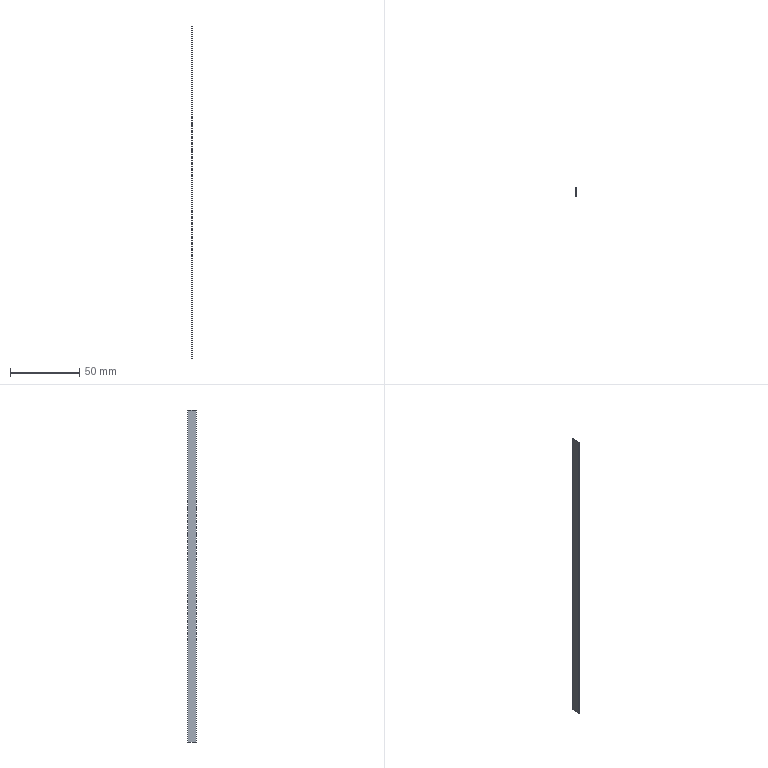Part | NX | features BREP 1 | 1 solid | 6 faces | box 0.3 x 6 x 240 mm | volume 432 mm3 | plane 6
STEP:
#1=CARTESIAN_POINT('',(0.15,-3.,-120.));
#2=VERTEX_POINT('',#1);
#3=CARTESIAN_POINT('',(0.15,3.,-120.));
#4=VERTEX_POINT('',#3);
#5=CARTESIAN_POINT('',(0.15,-3.,-120.));
#6=DIRECTION('',(0.,1.,0.));
#7=VECTOR('',#6,1000.);
#8=LINE('',#5,#7);
#9=EDGE_CURVE('',#2,#4,#8,.T.);
#10=ORIENTED_EDGE('',*,*,#9,.F.);
#11=CARTESIAN_POINT('',(-0.15,-3.,-120.));
#12=VERTEX_POINT('',#11);
#13=CARTESIAN_POINT('',(-0.15,-3.,-120.));
#14=DIRECTION('',(1.,0.,0.));
#15=VECTOR('',#14,1000.);
#16=LINE('',#13,#15);
#17=EDGE_CURVE('',#12,#2,#16,.T.);
#18=ORIENTED_EDGE('',*,*,#17,.F.);
#19=CARTESIAN_POINT('',(-0.15,3.,-120.));
#20=VERTEX_POINT('',#19);
#21=CARTESIAN_POINT('',(-0.15,-3.,-120.));
#22=DIRECTION('',(0.,-1.,0.));
#23=VECTOR('',#22,1000.);
#24=LINE('',#21,#23);
#25=EDGE_CURVE('',#20,#12,#24,.T.);
#26=ORIENTED_EDGE('',*,*,#25,.F.);
#27=CARTESIAN_POINT('',(-0.15,3.,-120.));
#28=DIRECTION('',(-1.,0.,0.));
#29=VECTOR('',#28,1000.);
#30=LINE('',#27,#29);
#31=EDGE_CURVE('',#4,#20,#30,.T.);
#32=ORIENTED_EDGE('',*,*,#31,.F.);
#33=EDGE_LOOP('',(#10,#18,#26,#32));
#34=FACE_BOUND('',#33,.T.);
#35=CARTESIAN_POINT('',(0.,0.,-120.));
#36=DIRECTION('',(0.,0.,-1.));
#37=DIRECTION('',(-1.,0.,0.));
#38=AXIS2_PLACEMENT_3D('',#35,#36,#37);
#39=PLANE('',#38);
#40=ADVANCED_FACE('',(#34),#39,.T.);
#41=CARTESIAN_POINT('',(0.15,-3.,120.));
#42=VERTEX_POINT('',#41);
#43=CARTESIAN_POINT('',(0.15,3.,120.));
#44=VERTEX_POINT('',#43);
#45=CARTESIAN_POINT('',(0.15,-3.,120.));
#46=DIRECTION('',(0.,1.,0.));
#47=VECTOR('',#46,1000.);
#48=LINE('',#45,#47);
#49=EDGE_CURVE('',#42,#44,#48,.T.);
#50=ORIENTED_EDGE('',*,*,#49,.T.);
#51=CARTESIAN_POINT('',(-0.15,3.,120.));
#52=VERTEX_POINT('',#51);
#53=CARTESIAN_POINT('',(-0.15,3.,120.));
#54=DIRECTION('',(-1.,0.,0.));
#55=VECTOR('',#54,1000.);
#56=LINE('',#53,#55);
#57=EDGE_CURVE('',#44,#52,#56,.T.);
#58=ORIENTED_EDGE('',*,*,#57,.T.);
#59=CARTESIAN_POINT('',(-0.15,-3.,120.));
#60=VERTEX_POINT('',#59);
#61=CARTESIAN_POINT('',(-0.15,-3.,120.));
#62=DIRECTION('',(0.,-1.,0.));
#63=VECTOR('',#62,1000.);
#64=LINE('',#61,#63);
#65=EDGE_CURVE('',#52,#60,#64,.T.);
#66=ORIENTED_EDGE('',*,*,#65,.T.);
#67=CARTESIAN_POINT('',(-0.15,-3.,120.));
#68=DIRECTION('',(1.,0.,0.));
#69=VECTOR('',#68,1000.);
#70=LINE('',#67,#69);
#71=EDGE_CURVE('',#60,#42,#70,.T.);
#72=ORIENTED_EDGE('',*,*,#71,.T.);
#73=EDGE_LOOP('',(#50,#58,#66,#72));
#74=FACE_BOUND('',#73,.T.);
#75=CARTESIAN_POINT('',(0.,0.,120.));
#76=DIRECTION('',(0.,0.,-1.));
#77=DIRECTION('',(-1.,0.,0.));
#78=AXIS2_PLACEMENT_3D('',#75,#76,#77);
#79=PLANE('',#78);
#80=ADVANCED_FACE('',(#74),#79,.F.);
#81=ORIENTED_EDGE('',*,*,#17,.T.);
#82=CARTESIAN_POINT('',(0.15,-3.,120.));
#83=DIRECTION('',(0.,0.,-1.));
#84=VECTOR('',#83,1000.);
#85=LINE('',#82,#84);
#86=EDGE_CURVE('',#42,#2,#85,.T.);
#87=ORIENTED_EDGE('',*,*,#86,.F.);
#88=ORIENTED_EDGE('',*,*,#71,.F.);
#89=CARTESIAN_POINT('',(-0.15,-3.,120.));
#90=DIRECTION('',(0.,0.,-1.));
#91=VECTOR('',#90,1000.);
#92=LINE('',#89,#91);
#93=EDGE_CURVE('',#60,#12,#92,.T.);
#94=ORIENTED_EDGE('',*,*,#93,.T.);
#95=EDGE_LOOP('',(#81,#87,#88,#94));
#96=FACE_BOUND('',#95,.T.);
#97=CARTESIAN_POINT('',(-0.15,-3.,120.));
#98=DIRECTION('',(0.,1.,0.));
#99=DIRECTION('',(0.,0.,1.));
#100=AXIS2_PLACEMENT_3D('',#97,#98,#99);
#101=PLANE('',#100);
#102=ADVANCED_FACE('',(#96),#101,.F.);
#103=ORIENTED_EDGE('',*,*,#25,.T.);
#104=ORIENTED_EDGE('',*,*,#93,.F.);
#105=ORIENTED_EDGE('',*,*,#65,.F.);
#106=CARTESIAN_POINT('',(-0.15,3.,120.));
#107=DIRECTION('',(0.,0.,-1.));
#108=VECTOR('',#107,1000.);
#109=LINE('',#106,#108);
#110=EDGE_CURVE('',#52,#20,#109,.T.);
#111=ORIENTED_EDGE('',*,*,#110,.T.);
#112=EDGE_LOOP('',(#103,#104,#105,#111));
#113=FACE_BOUND('',#112,.T.);
#114=CARTESIAN_POINT('',(-0.15,-3.,120.));
#115=DIRECTION('',(1.,0.,0.));
#116=DIRECTION('',(0.,0.,-1.));
#117=AXIS2_PLACEMENT_3D('',#114,#115,#116);
#118=PLANE('',#117);
#119=ADVANCED_FACE('',(#113),#118,.F.);
#120=ORIENTED_EDGE('',*,*,#31,.T.);
#121=ORIENTED_EDGE('',*,*,#110,.F.);
#122=ORIENTED_EDGE('',*,*,#57,.F.);
#123=CARTESIAN_POINT('',(0.15,3.,120.));
#124=DIRECTION('',(0.,0.,-1.));
#125=VECTOR('',#124,1000.);
#126=LINE('',#123,#125);
#127=EDGE_CURVE('',#44,#4,#126,.T.);
#128=ORIENTED_EDGE('',*,*,#127,.T.);
#129=EDGE_LOOP('',(#120,#121,#122,#128));
#130=FACE_BOUND('',#129,.T.);
#131=CARTESIAN_POINT('',(-0.15,3.,120.));
#132=DIRECTION('',(0.,-1.,0.));
#133=DIRECTION('',(0.,0.,-1.));
#134=AXIS2_PLACEMENT_3D('',#131,#132,#133);
#135=PLANE('',#134);
#136=ADVANCED_FACE('',(#130),#135,.F.);
#137=ORIENTED_EDGE('',*,*,#9,.T.);
#138=ORIENTED_EDGE('',*,*,#127,.F.);
#139=ORIENTED_EDGE('',*,*,#49,.F.);
#140=ORIENTED_EDGE('',*,*,#86,.T.);
#141=EDGE_LOOP('',(#137,#138,#139,#140));
#142=FACE_BOUND('',#141,.T.);
#143=CARTESIAN_POINT('',(0.15,-3.,120.));
#144=DIRECTION('',(-1.,0.,0.));
#145=DIRECTION('',(0.,0.,1.));
#146=AXIS2_PLACEMENT_3D('',#143,#144,#145);
#147=PLANE('',#146);
#148=ADVANCED_FACE('',(#142),#147,.F.);
#149=CLOSED_SHELL('',(#40,#80,#102,#119,#136,#148));
#150=MANIFOLD_SOLID_BREP('',#149);
#151=(LENGTH_UNIT()NAMED_UNIT(*)SI_UNIT(.MILLI.,.METRE.));
#152=UNCERTAINTY_MEASURE_WITH_UNIT(LENGTH_MEASURE(0.00001),#151,'','');
#153=(NAMED_UNIT(*)PLANE_ANGLE_UNIT()SI_UNIT($,.RADIAN.));
#154=(NAMED_UNIT(*)SI_UNIT($,.STERADIAN.)SOLID_ANGLE_UNIT());
#155=(GEOMETRIC_REPRESENTATION_CONTEXT(3)GLOBAL_UNCERTAINTY_ASSIGNED_CONTEXT((#152))GLOBAL_UNIT_ASSIGNED_CONTEXT((#151,#153,#154))REPRESENTATION_CONTEXT('',''));
#156=ADVANCED_BREP_SHAPE_REPRESENTATION('',(#150),#155);